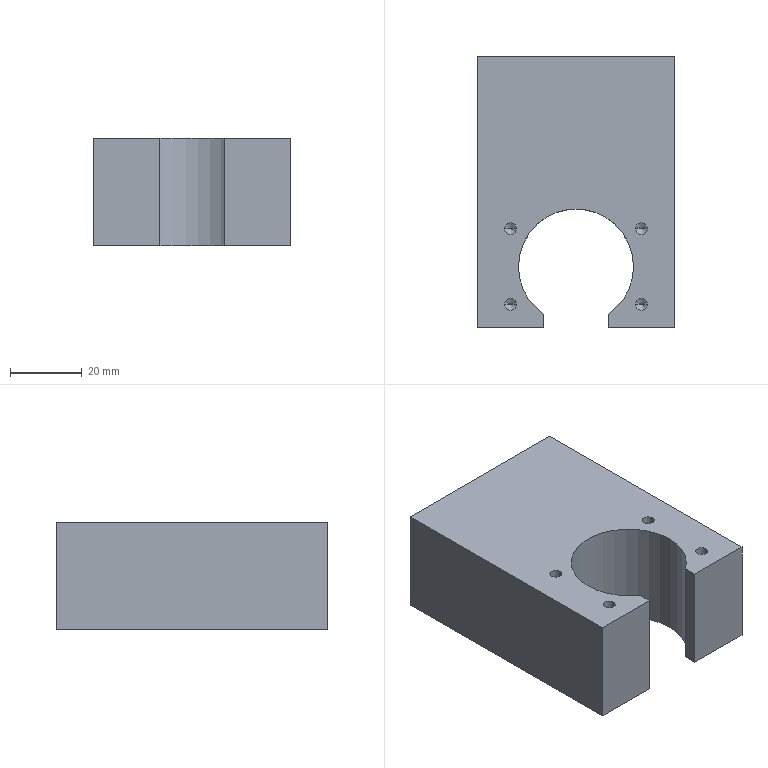Part | SolidWorks | features HoleWzd 2, 3DProfileFeature 1, Extrusion 1 | 1 solid | 52 faces | box 55 x 75.5 x 30 mm | volume 98100 mm3 | cone 24 | cylinder 19 | plane 9 | commonest cylinder face diameters 3.3 x8 5 x8 32 x3
STEP:
#1=CARTESIAN_POINT('',(-20.5,57.975,5.5));
#2=VERTEX_POINT('',#1);
#3=CARTESIAN_POINT('',(-20.5,57.975,10.5));
#4=VERTEX_POINT('',#3);
#5=CARTESIAN_POINT('',(-20.5,57.975,8.));
#6=DIRECTION('',(0.,1.,0.));
#7=DIRECTION('',(0.,0.,1.));
#8=AXIS2_PLACEMENT_3D('',#5,#6,#7);
#9=CIRCLE('',#8,2.5);
#10=EDGE_CURVE('',#2,#4,#9,.T.);
#11=ORIENTED_EDGE('',*,*,#10,.F.);
#12=CARTESIAN_POINT('',(-20.5,58.5,4.975));
#13=VERTEX_POINT('',#12);
#14=CARTESIAN_POINT('',(-20.5,58.5,4.975));
#15=DIRECTION('',(0.,0.7071,-0.7071));
#16=VECTOR('',#15,1000.);
#17=LINE('',#14,#16);
#18=EDGE_CURVE('',#2,#13,#17,.T.);
#19=ORIENTED_EDGE('',*,*,#18,.T.);
#20=CARTESIAN_POINT('',(-20.5,58.5,11.025));
#21=VERTEX_POINT('',#20);
#22=CARTESIAN_POINT('',(-20.5,58.5,8.));
#23=DIRECTION('',(0.,1.,0.));
#24=DIRECTION('',(0.,0.,1.));
#25=AXIS2_PLACEMENT_3D('',#22,#23,#24);
#26=CIRCLE('',#25,3.025);
#27=EDGE_CURVE('',#13,#21,#26,.T.);
#28=ORIENTED_EDGE('',*,*,#27,.T.);
#29=CARTESIAN_POINT('',(-20.5,58.5,11.025));
#30=DIRECTION('',(0.,0.7071,0.7071));
#31=VECTOR('',#30,1000.);
#32=LINE('',#29,#31);
#33=EDGE_CURVE('',#4,#21,#32,.T.);
#34=ORIENTED_EDGE('',*,*,#33,.F.);
#35=EDGE_LOOP('',(#11,#19,#28,#34));
#36=FACE_OUTER_BOUND('',#35,.T.);
#37=CARTESIAN_POINT('',(-20.5,58.5,8.));
#38=DIRECTION('',(0.,1.,0.));
#39=DIRECTION('',(0.,0.,1.));
#40=AXIS2_PLACEMENT_3D('',#37,#38,#39);
#41=CONICAL_SURFACE('',#40,3.025,0.7854);
#42=ADVANCED_FACE('',(#36),#41,.F.);
#43=CARTESIAN_POINT('',(-20.5,46.5,5.5));
#44=VERTEX_POINT('',#43);
#45=CARTESIAN_POINT('',(-20.5,46.5,10.5));
#46=VERTEX_POINT('',#45);
#47=CARTESIAN_POINT('',(-20.5,46.5,8.));
#48=DIRECTION('',(0.,1.,0.));
#49=DIRECTION('',(0.,0.,1.));
#50=AXIS2_PLACEMENT_3D('',#47,#48,#49);
#51=CIRCLE('',#50,2.5);
#52=EDGE_CURVE('',#44,#46,#51,.T.);
#53=ORIENTED_EDGE('',*,*,#52,.F.);
#54=CARTESIAN_POINT('',(-20.5,58.5,5.5));
#55=DIRECTION('',(0.,1.,0.));
#56=VECTOR('',#55,1000.);
#57=LINE('',#54,#56);
#58=EDGE_CURVE('',#44,#2,#57,.T.);
#59=ORIENTED_EDGE('',*,*,#58,.T.);
#60=ORIENTED_EDGE('',*,*,#10,.T.);
#61=CARTESIAN_POINT('',(-20.5,58.5,10.5));
#62=DIRECTION('',(0.,1.,0.));
#63=VECTOR('',#62,1000.);
#64=LINE('',#61,#63);
#65=EDGE_CURVE('',#46,#4,#64,.T.);
#66=ORIENTED_EDGE('',*,*,#65,.F.);
#67=EDGE_LOOP('',(#53,#59,#60,#66));
#68=FACE_OUTER_BOUND('',#67,.T.);
#69=CARTESIAN_POINT('',(-20.5,58.5,8.));
#70=DIRECTION('',(0.,1.,0.));
#71=DIRECTION('',(0.,0.,1.));
#72=AXIS2_PLACEMENT_3D('',#69,#70,#71);
#73=CYLINDRICAL_SURFACE('',#72,2.5);
#74=ADVANCED_FACE('',(#68),#73,.F.);
#75=CARTESIAN_POINT('',(-20.5,44.998,8.));
#76=VERTEX_POINT('',#75);
#77=CARTESIAN_POINT('',(-20.5,46.5,10.5));
#78=DIRECTION('',(0.,0.515,0.8572));
#79=VECTOR('',#78,1000.);
#80=LINE('',#77,#79);
#81=EDGE_CURVE('',#76,#46,#80,.T.);
#82=ORIENTED_EDGE('',*,*,#81,.F.);
#83=CARTESIAN_POINT('',(-20.5,46.5,5.5));
#84=DIRECTION('',(0.,0.515,-0.8572));
#85=VECTOR('',#84,1000.);
#86=LINE('',#83,#85);
#87=EDGE_CURVE('',#76,#44,#86,.T.);
#88=ORIENTED_EDGE('',*,*,#87,.T.);
#89=ORIENTED_EDGE('',*,*,#52,.T.);
#90=EDGE_LOOP('',(#82,#88,#89));
#91=FACE_OUTER_BOUND('',#90,.T.);
#92=CARTESIAN_POINT('',(-20.5,46.5,8.));
#93=DIRECTION('',(0.,1.,0.));
#94=DIRECTION('',(0.,0.,1.));
#95=AXIS2_PLACEMENT_3D('',#92,#93,#94);
#96=CONICAL_SURFACE('',#95,2.5,1.03);
#97=ADVANCED_FACE('',(#91),#96,.F.);
#98=CARTESIAN_POINT('',(-20.5,57.975,-10.5));
#99=VERTEX_POINT('',#98);
#100=CARTESIAN_POINT('',(-20.5,57.975,-5.5));
#101=VERTEX_POINT('',#100);
#102=CARTESIAN_POINT('',(-20.5,57.975,-8.));
#103=DIRECTION('',(0.,1.,0.));
#104=DIRECTION('',(0.,0.,1.));
#105=AXIS2_PLACEMENT_3D('',#102,#103,#104);
#106=CIRCLE('',#105,2.5);
#107=EDGE_CURVE('',#99,#101,#106,.T.);
#108=ORIENTED_EDGE('',*,*,#107,.F.);
#109=CARTESIAN_POINT('',(-20.5,58.5,-11.025));
#110=VERTEX_POINT('',#109);
#111=CARTESIAN_POINT('',(-20.5,58.5,-11.025));
#112=DIRECTION('',(0.,0.7071,-0.7071));
#113=VECTOR('',#112,1000.);
#114=LINE('',#111,#113);
#115=EDGE_CURVE('',#99,#110,#114,.T.);
#116=ORIENTED_EDGE('',*,*,#115,.T.);
#117=CARTESIAN_POINT('',(-20.5,58.5,-4.975));
#118=VERTEX_POINT('',#117);
#119=CARTESIAN_POINT('',(-20.5,58.5,-8.));
#120=DIRECTION('',(0.,1.,0.));
#121=DIRECTION('',(0.,0.,1.));
#122=AXIS2_PLACEMENT_3D('',#119,#120,#121);
#123=CIRCLE('',#122,3.025);
#124=EDGE_CURVE('',#110,#118,#123,.T.);
#125=ORIENTED_EDGE('',*,*,#124,.T.);
#126=CARTESIAN_POINT('',(-20.5,58.5,-4.975));
#127=DIRECTION('',(0.,0.7071,0.7071));
#128=VECTOR('',#127,1000.);
#129=LINE('',#126,#128);
#130=EDGE_CURVE('',#101,#118,#129,.T.);
#131=ORIENTED_EDGE('',*,*,#130,.F.);
#132=EDGE_LOOP('',(#108,#116,#125,#131));
#133=FACE_OUTER_BOUND('',#132,.T.);
#134=CARTESIAN_POINT('',(-20.5,58.5,-8.));
#135=DIRECTION('',(0.,1.,0.));
#136=DIRECTION('',(0.,0.,1.));
#137=AXIS2_PLACEMENT_3D('',#134,#135,#136);
#138=CONICAL_SURFACE('',#137,3.025,0.7854);
#139=ADVANCED_FACE('',(#133),#138,.F.);
#140=CARTESIAN_POINT('',(-20.5,46.5,-10.5));
#141=VERTEX_POINT('',#140);
#142=CARTESIAN_POINT('',(-20.5,46.5,-5.5));
#143=VERTEX_POINT('',#142);
#144=CARTESIAN_POINT('',(-20.5,46.5,-8.));
#145=DIRECTION('',(0.,1.,0.));
#146=DIRECTION('',(0.,0.,1.));
#147=AXIS2_PLACEMENT_3D('',#144,#145,#146);
#148=CIRCLE('',#147,2.5);
#149=EDGE_CURVE('',#141,#143,#148,.T.);
#150=ORIENTED_EDGE('',*,*,#149,.F.);
#151=CARTESIAN_POINT('',(-20.5,58.5,-10.5));
#152=DIRECTION('',(0.,1.,0.));
#153=VECTOR('',#152,1000.);
#154=LINE('',#151,#153);
#155=EDGE_CURVE('',#141,#99,#154,.T.);
#156=ORIENTED_EDGE('',*,*,#155,.T.);
#157=ORIENTED_EDGE('',*,*,#107,.T.);
#158=CARTESIAN_POINT('',(-20.5,58.5,-5.5));
#159=DIRECTION('',(0.,1.,0.));
#160=VECTOR('',#159,1000.);
#161=LINE('',#158,#160);
#162=EDGE_CURVE('',#143,#101,#161,.T.);
#163=ORIENTED_EDGE('',*,*,#162,.F.);
#164=EDGE_LOOP('',(#150,#156,#157,#163));
#165=FACE_OUTER_BOUND('',#164,.T.);
#166=CARTESIAN_POINT('',(-20.5,58.5,-8.));
#167=DIRECTION('',(0.,1.,0.));
#168=DIRECTION('',(0.,0.,1.));
#169=AXIS2_PLACEMENT_3D('',#166,#167,#168);
#170=CYLINDRICAL_SURFACE('',#169,2.5);
#171=ADVANCED_FACE('',(#165),#170,.F.);
#172=CARTESIAN_POINT('',(-20.5,44.998,-8.));
#173=VERTEX_POINT('',#172);
#174=CARTESIAN_POINT('',(-20.5,46.5,-5.5));
#175=DIRECTION('',(0.,0.515,0.8572));
#176=VECTOR('',#175,1000.);
#177=LINE('',#174,#176);
#178=EDGE_CURVE('',#173,#143,#177,.T.);
#179=ORIENTED_EDGE('',*,*,#178,.F.);
#180=CARTESIAN_POINT('',(-20.5,46.5,-10.5));
#181=DIRECTION('',(0.,0.515,-0.8572));
#182=VECTOR('',#181,1000.);
#183=LINE('',#180,#182);
#184=EDGE_CURVE('',#173,#141,#183,.T.);
#185=ORIENTED_EDGE('',*,*,#184,.T.);
#186=ORIENTED_EDGE('',*,*,#149,.T.);
#187=EDGE_LOOP('',(#179,#185,#186));
#188=FACE_OUTER_BOUND('',#187,.T.);
#189=CARTESIAN_POINT('',(-20.5,46.5,-8.));
#190=DIRECTION('',(0.,1.,0.));
#191=DIRECTION('',(0.,0.,1.));
#192=AXIS2_PLACEMENT_3D('',#189,#190,#191);
#193=CONICAL_SURFACE('',#192,2.5,1.03);
#194=ADVANCED_FACE('',(#188),#193,.F.);
#195=CARTESIAN_POINT('',(20.5,57.975,-10.5));
#196=VERTEX_POINT('',#195);
#197=CARTESIAN_POINT('',(20.5,57.975,-5.5));
#198=VERTEX_POINT('',#197);
#199=CARTESIAN_POINT('',(20.5,57.975,-8.));
#200=DIRECTION('',(0.,1.,0.));
#201=DIRECTION('',(0.,0.,1.));
#202=AXIS2_PLACEMENT_3D('',#199,#200,#201);
#203=CIRCLE('',#202,2.5);
#204=EDGE_CURVE('',#196,#198,#203,.T.);
#205=ORIENTED_EDGE('',*,*,#204,.F.);
#206=CARTESIAN_POINT('',(20.5,58.5,-11.025));
#207=VERTEX_POINT('',#206);
#208=CARTESIAN_POINT('',(20.5,58.5,-11.025));
#209=DIRECTION('',(0.,0.7071,-0.7071));
#210=VECTOR('',#209,1000.);
#211=LINE('',#208,#210);
#212=EDGE_CURVE('',#196,#207,#211,.T.);
#213=ORIENTED_EDGE('',*,*,#212,.T.);
#214=CARTESIAN_POINT('',(20.5,58.5,-4.975));
#215=VERTEX_POINT('',#214);
#216=CARTESIAN_POINT('',(20.5,58.5,-8.));
#217=DIRECTION('',(0.,1.,0.));
#218=DIRECTION('',(0.,0.,1.));
#219=AXIS2_PLACEMENT_3D('',#216,#217,#218);
#220=CIRCLE('',#219,3.025);
#221=EDGE_CURVE('',#207,#215,#220,.T.);
#222=ORIENTED_EDGE('',*,*,#221,.T.);
#223=CARTESIAN_POINT('',(20.5,58.5,-4.975));
#224=DIRECTION('',(0.,0.7071,0.7071));
#225=VECTOR('',#224,1000.);
#226=LINE('',#223,#225);
#227=EDGE_CURVE('',#198,#215,#226,.T.);
#228=ORIENTED_EDGE('',*,*,#227,.F.);
#229=EDGE_LOOP('',(#205,#213,#222,#228));
#230=FACE_OUTER_BOUND('',#229,.T.);
#231=CARTESIAN_POINT('',(20.5,58.5,-8.));
#232=DIRECTION('',(0.,1.,0.));
#233=DIRECTION('',(0.,0.,1.));
#234=AXIS2_PLACEMENT_3D('',#231,#232,#233);
#235=CONICAL_SURFACE('',#234,3.025,0.7854);
#236=ADVANCED_FACE('',(#230),#235,.F.);
#237=CARTESIAN_POINT('',(20.5,46.5,-10.5));
#238=VERTEX_POINT('',#237);
#239=CARTESIAN_POINT('',(20.5,46.5,-5.5));
#240=VERTEX_POINT('',#239);
#241=CARTESIAN_POINT('',(20.5,46.5,-8.));
#242=DIRECTION('',(0.,1.,0.));
#243=DIRECTION('',(0.,0.,1.));
#244=AXIS2_PLACEMENT_3D('',#241,#242,#243);
#245=CIRCLE('',#244,2.5);
#246=EDGE_CURVE('',#238,#240,#245,.T.);
#247=ORIENTED_EDGE('',*,*,#246,.F.);
#248=CARTESIAN_POINT('',(20.5,58.5,-10.5));
#249=DIRECTION('',(0.,1.,0.));
#250=VECTOR('',#249,1000.);
#251=LINE('',#248,#250);
#252=EDGE_CURVE('',#238,#196,#251,.T.);
#253=ORIENTED_EDGE('',*,*,#252,.T.);
#254=ORIENTED_EDGE('',*,*,#204,.T.);
#255=CARTESIAN_POINT('',(20.5,58.5,-5.5));
#256=DIRECTION('',(0.,1.,0.));
#257=VECTOR('',#256,1000.);
#258=LINE('',#255,#257);
#259=EDGE_CURVE('',#240,#198,#258,.T.);
#260=ORIENTED_EDGE('',*,*,#259,.F.);
#261=EDGE_LOOP('',(#247,#253,#254,#260));
#262=FACE_OUTER_BOUND('',#261,.T.);
#263=CARTESIAN_POINT('',(20.5,58.5,-8.));
#264=DIRECTION('',(0.,1.,0.));
#265=DIRECTION('',(0.,0.,1.));
#266=AXIS2_PLACEMENT_3D('',#263,#264,#265);
#267=CYLINDRICAL_SURFACE('',#266,2.5);
#268=ADVANCED_FACE('',(#262),#267,.F.);
#269=CARTESIAN_POINT('',(20.5,44.998,-8.));
#270=VERTEX_POINT('',#269);
#271=CARTESIAN_POINT('',(20.5,46.5,-5.5));
#272=DIRECTION('',(0.,0.515,0.8572));
#273=VECTOR('',#272,1000.);
#274=LINE('',#271,#273);
#275=EDGE_CURVE('',#270,#240,#274,.T.);
#276=ORIENTED_EDGE('',*,*,#275,.F.);
#277=CARTESIAN_POINT('',(20.5,46.5,-10.5));
#278=DIRECTION('',(0.,0.515,-0.8572));
#279=VECTOR('',#278,1000.);
#280=LINE('',#277,#279);
#281=EDGE_CURVE('',#270,#238,#280,.T.);
#282=ORIENTED_EDGE('',*,*,#281,.T.);
#283=ORIENTED_EDGE('',*,*,#246,.T.);
#284=EDGE_LOOP('',(#276,#282,#283));
#285=FACE_OUTER_BOUND('',#284,.T.);
#286=CARTESIAN_POINT('',(20.5,46.5,-8.));
#287=DIRECTION('',(0.,1.,0.));
#288=DIRECTION('',(0.,0.,1.));
#289=AXIS2_PLACEMENT_3D('',#286,#287,#288);
#290=CONICAL_SURFACE('',#289,2.5,1.03);
#291=ADVANCED_FACE('',(#285),#290,.F.);
#292=CARTESIAN_POINT('',(20.5,57.975,5.5));
#293=VERTEX_POINT('',#292);
#294=CARTESIAN_POINT('',(20.5,57.975,10.5));
#295=VERTEX_POINT('',#294);
#296=CARTESIAN_POINT('',(20.5,57.975,8.));
#297=DIRECTION('',(0.,1.,0.));
#298=DIRECTION('',(0.,0.,1.));
#299=AXIS2_PLACEMENT_3D('',#296,#297,#298);
#300=CIRCLE('',#299,2.5);
#301=EDGE_CURVE('',#293,#295,#300,.T.);
#302=ORIENTED_EDGE('',*,*,#301,.F.);
#303=CARTESIAN_POINT('',(20.5,58.5,4.975));
#304=VERTEX_POINT('',#303);
#305=CARTESIAN_POINT('',(20.5,58.5,4.975));
#306=DIRECTION('',(0.,0.7071,-0.7071));
#307=VECTOR('',#306,1000.);
#308=LINE('',#305,#307);
#309=EDGE_CURVE('',#293,#304,#308,.T.);
#310=ORIENTED_EDGE('',*,*,#309,.T.);
#311=CARTESIAN_POINT('',(20.5,58.5,11.025));
#312=VERTEX_POINT('',#311);
#313=CARTESIAN_POINT('',(20.5,58.5,8.));
#314=DIRECTION('',(0.,1.,0.));
#315=DIRECTION('',(0.,0.,1.));
#316=AXIS2_PLACEMENT_3D('',#313,#314,#315);
#317=CIRCLE('',#316,3.025);
#318=EDGE_CURVE('',#304,#312,#317,.T.);
#319=ORIENTED_EDGE('',*,*,#318,.T.);
#320=CARTESIAN_POINT('',(20.5,58.5,11.025));
#321=DIRECTION('',(0.,0.7071,0.7071));
#322=VECTOR('',#321,1000.);
#323=LINE('',#320,#322);
#324=EDGE_CURVE('',#295,#312,#323,.T.);
#325=ORIENTED_EDGE('',*,*,#324,.F.);
#326=EDGE_LOOP('',(#302,#310,#319,#325));
#327=FACE_OUTER_BOUND('',#326,.T.);
#328=CARTESIAN_POINT('',(20.5,58.5,8.));
#329=DIRECTION('',(0.,1.,0.));
#330=DIRECTION('',(0.,0.,1.));
#331=AXIS2_PLACEMENT_3D('',#328,#329,#330);
#332=CONICAL_SURFACE('',#331,3.025,0.7854);
#333=ADVANCED_FACE('',(#327),#332,.F.);
#334=CARTESIAN_POINT('',(20.5,46.5,5.5));
#335=VERTEX_POINT('',#334);
#336=CARTESIAN_POINT('',(20.5,46.5,10.5));
#337=VERTEX_POINT('',#336);
#338=CARTESIAN_POINT('',(20.5,46.5,8.));
#339=DIRECTION('',(0.,1.,0.));
#340=DIRECTION('',(0.,0.,1.));
#341=AXIS2_PLACEMENT_3D('',#338,#339,#340);
#342=CIRCLE('',#341,2.5);
#343=EDGE_CURVE('',#335,#337,#342,.T.);
#344=ORIENTED_EDGE('',*,*,#343,.F.);
#345=CARTESIAN_POINT('',(20.5,58.5,5.5));
#346=DIRECTION('',(0.,1.,0.));
#347=VECTOR('',#346,1000.);
#348=LINE('',#345,#347);
#349=EDGE_CURVE('',#335,#293,#348,.T.);
#350=ORIENTED_EDGE('',*,*,#349,.T.);
#351=ORIENTED_EDGE('',*,*,#301,.T.);
#352=CARTESIAN_POINT('',(20.5,58.5,10.5));
#353=DIRECTION('',(0.,1.,0.));
#354=VECTOR('',#353,1000.);
#355=LINE('',#352,#354);
#356=EDGE_CURVE('',#337,#295,#355,.T.);
#357=ORIENTED_EDGE('',*,*,#356,.F.);
#358=EDGE_LOOP('',(#344,#350,#351,#357));
#359=FACE_OUTER_BOUND('',#358,.T.);
#360=CARTESIAN_POINT('',(20.5,58.5,8.));
#361=DIRECTION('',(0.,1.,0.));
#362=DIRECTION('',(0.,0.,1.));
#363=AXIS2_PLACEMENT_3D('',#360,#361,#362);
#364=CYLINDRICAL_SURFACE('',#363,2.5);
#365=ADVANCED_FACE('',(#359),#364,.F.);
#366=CARTESIAN_POINT('',(20.5,44.998,8.));
#367=VERTEX_POINT('',#366);
#368=CARTESIAN_POINT('',(20.5,46.5,10.5));
#369=DIRECTION('',(0.,0.515,0.8572));
#370=VECTOR('',#369,1000.);
#371=LINE('',#368,#370);
#372=EDGE_CURVE('',#367,#337,#371,.T.);
#373=ORIENTED_EDGE('',*,*,#372,.F.);
#374=CARTESIAN_POINT('',(20.5,46.5,5.5));
#375=DIRECTION('',(0.,0.515,-0.8572));
#376=VECTOR('',#375,1000.);
#377=LINE('',#374,#376);
#378=EDGE_CURVE('',#367,#335,#377,.T.);
#379=ORIENTED_EDGE('',*,*,#378,.T.);
#380=ORIENTED_EDGE('',*,*,#343,.T.);
#381=EDGE_LOOP('',(#373,#379,#380));
#382=FACE_OUTER_BOUND('',#381,.T.);
#383=CARTESIAN_POINT('',(20.5,46.5,8.));
#384=DIRECTION('',(0.,1.,0.));
#385=DIRECTION('',(0.,0.,1.));
#386=AXIS2_PLACEMENT_3D('',#383,#384,#385);
#387=CONICAL_SURFACE('',#386,2.5,1.03);
#388=ADVANCED_FACE('',(#382),#387,.F.);
#389=CARTESIAN_POINT('',(16.537,10.5,5.5));
#390=VERTEX_POINT('',#389);
#391=CARTESIAN_POINT('',(19.837,10.5,5.5));
#392=VERTEX_POINT('',#391);
#393=CARTESIAN_POINT('',(18.187,10.5,5.5));
#394=DIRECTION('',(0.,0.,1.));
#395=DIRECTION('',(1.,0.,0.));
#396=AXIS2_PLACEMENT_3D('',#393,#394,#395);
#397=CIRCLE('',#396,1.65);
#398=EDGE_CURVE('',#390,#392,#397,.T.);
#399=ORIENTED_EDGE('',*,*,#398,.F.);
#400=CARTESIAN_POINT('',(16.537,10.5,15.));
#401=VERTEX_POINT('',#400);
#402=CARTESIAN_POINT('',(16.537,10.5,15.));
#403=DIRECTION('',(0.,0.,1.));
#404=VECTOR('',#403,1000.);
#405=LINE('',#402,#404);
#406=EDGE_CURVE('',#390,#401,#405,.T.);
#407=ORIENTED_EDGE('',*,*,#406,.T.);
#408=CARTESIAN_POINT('',(19.837,10.5,15.));
#409=VERTEX_POINT('',#408);
#410=CARTESIAN_POINT('',(18.187,10.5,15.));
#411=DIRECTION('',(0.,0.,1.));
#412=DIRECTION('',(1.,0.,0.));
#413=AXIS2_PLACEMENT_3D('',#410,#411,#412);
#414=CIRCLE('',#413,1.65);
#415=EDGE_CURVE('',#401,#409,#414,.T.);
#416=ORIENTED_EDGE('',*,*,#415,.T.);
#417=CARTESIAN_POINT('',(19.837,10.5,15.));
#418=DIRECTION('',(0.,0.,1.));
#419=VECTOR('',#418,1000.);
#420=LINE('',#417,#419);
#421=EDGE_CURVE('',#392,#409,#420,.T.);
#422=ORIENTED_EDGE('',*,*,#421,.F.);
#423=EDGE_LOOP('',(#399,#407,#416,#422));
#424=FACE_OUTER_BOUND('',#423,.T.);
#425=CARTESIAN_POINT('',(18.187,10.5,15.));
#426=DIRECTION('',(0.,0.,1.));
#427=DIRECTION('',(1.,0.,0.));
#428=AXIS2_PLACEMENT_3D('',#425,#426,#427);
#429=CYLINDRICAL_SURFACE('',#428,1.65);
#430=ADVANCED_FACE('',(#424),#429,.F.);
#431=CARTESIAN_POINT('',(18.187,10.5,4.509));
#432=VERTEX_POINT('',#431);
#433=CARTESIAN_POINT('',(19.837,10.5,5.5));
#434=DIRECTION('',(0.8572,0.,0.515));
#435=VECTOR('',#434,1000.);
#436=LINE('',#433,#435);
#437=EDGE_CURVE('',#432,#392,#436,.T.);
#438=ORIENTED_EDGE('',*,*,#437,.F.);
#439=CARTESIAN_POINT('',(16.537,10.5,5.5));
#440=DIRECTION('',(-0.8572,0.,0.515));
#441=VECTOR('',#440,1000.);
#442=LINE('',#439,#441);
#443=EDGE_CURVE('',#432,#390,#442,.T.);
#444=ORIENTED_EDGE('',*,*,#443,.T.);
#445=ORIENTED_EDGE('',*,*,#398,.T.);
#446=EDGE_LOOP('',(#438,#444,#445));
#447=FACE_OUTER_BOUND('',#446,.T.);
#448=CARTESIAN_POINT('',(18.187,10.5,5.5));
#449=DIRECTION('',(0.,0.,1.));
#450=DIRECTION('',(1.,0.,0.));
#451=AXIS2_PLACEMENT_3D('',#448,#449,#450);
#452=CONICAL_SURFACE('',#451,1.65,1.03);
#453=ADVANCED_FACE('',(#447),#452,.F.);
#454=CARTESIAN_POINT('',(16.537,-10.5,5.5));
#455=VERTEX_POINT('',#454);
#456=CARTESIAN_POINT('',(19.837,-10.5,5.5));
#457=VERTEX_POINT('',#456);
#458=CARTESIAN_POINT('',(18.187,-10.5,5.5));
#459=DIRECTION('',(0.,0.,1.));
#460=DIRECTION('',(1.,0.,0.));
#461=AXIS2_PLACEMENT_3D('',#458,#459,#460);
#462=CIRCLE('',#461,1.65);
#463=EDGE_CURVE('',#455,#457,#462,.T.);
#464=ORIENTED_EDGE('',*,*,#463,.F.);
#465=CARTESIAN_POINT('',(16.537,-10.5,15.));
#466=VERTEX_POINT('',#465);
#467=CARTESIAN_POINT('',(16.537,-10.5,15.));
#468=DIRECTION('',(0.,0.,1.));
#469=VECTOR('',#468,1000.);
#470=LINE('',#467,#469);
#471=EDGE_CURVE('',#455,#466,#470,.T.);
#472=ORIENTED_EDGE('',*,*,#471,.T.);
#473=CARTESIAN_POINT('',(19.837,-10.5,15.));
#474=VERTEX_POINT('',#473);
#475=CARTESIAN_POINT('',(18.187,-10.5,15.));
#476=DIRECTION('',(0.,0.,1.));
#477=DIRECTION('',(1.,0.,0.));
#478=AXIS2_PLACEMENT_3D('',#475,#476,#477);
#479=CIRCLE('',#478,1.65);
#480=EDGE_CURVE('',#466,#474,#479,.T.);
#481=ORIENTED_EDGE('',*,*,#480,.T.);
#482=CARTESIAN_POINT('',(19.837,-10.5,15.));
#483=DIRECTION('',(0.,0.,1.));
#484=VECTOR('',#483,1000.);
#485=LINE('',#482,#484);
#486=EDGE_CURVE('',#457,#474,#485,.T.);
#487=ORIENTED_EDGE('',*,*,#486,.F.);
#488=EDGE_LOOP('',(#464,#472,#481,#487));
#489=FACE_OUTER_BOUND('',#488,.T.);
#490=CARTESIAN_POINT('',(18.187,-10.5,15.));
#491=DIRECTION('',(0.,0.,1.));
#492=DIRECTION('',(1.,0.,0.));
#493=AXIS2_PLACEMENT_3D('',#490,#491,#492);
#494=CYLINDRICAL_SURFACE('',#493,1.65);
#495=ADVANCED_FACE('',(#489),#494,.F.);
#496=CARTESIAN_POINT('',(18.187,-10.5,4.509));
#497=VERTEX_POINT('',#496);
#498=CARTESIAN_POINT('',(19.837,-10.5,5.5));
#499=DIRECTION('',(0.8572,0.,0.515));
#500=VECTOR('',#499,1000.);
#501=LINE('',#498,#500);
#502=EDGE_CURVE('',#497,#457,#501,.T.);
#503=ORIENTED_EDGE('',*,*,#502,.F.);
#504=CARTESIAN_POINT('',(16.537,-10.5,5.5));
#505=DIRECTION('',(-0.8572,0.,0.515));
#506=VECTOR('',#505,1000.);
#507=LINE('',#504,#506);
#508=EDGE_CURVE('',#497,#455,#507,.T.);
#509=ORIENTED_EDGE('',*,*,#508,.T.);
#510=ORIENTED_EDGE('',*,*,#463,.T.);
#511=EDGE_LOOP('',(#503,#509,#510));
#512=FACE_OUTER_BOUND('',#511,.T.);
#513=CARTESIAN_POINT('',(18.187,-10.5,5.5));
#514=DIRECTION('',(0.,0.,1.));
#515=DIRECTION('',(1.,0.,0.));
#516=AXIS2_PLACEMENT_3D('',#513,#514,#515);
#517=CONICAL_SURFACE('',#516,1.65,1.03);
#518=ADVANCED_FACE('',(#512),#517,.F.);
#519=CARTESIAN_POINT('',(-19.837,-10.5,5.5));
#520=VERTEX_POINT('',#519);
#521=CARTESIAN_POINT('',(-16.537,-10.5,5.5));
#522=VERTEX_POINT('',#521);
#523=CARTESIAN_POINT('',(-18.187,-10.5,5.5));
#524=DIRECTION('',(0.,0.,1.));
#525=DIRECTION('',(1.,0.,0.));
#526=AXIS2_PLACEMENT_3D('',#523,#524,#525);
#527=CIRCLE('',#526,1.65);
#528=EDGE_CURVE('',#520,#522,#527,.T.);
#529=ORIENTED_EDGE('',*,*,#528,.F.);
#530=CARTESIAN_POINT('',(-19.837,-10.5,15.));
#531=VERTEX_POINT('',#530);
#532=CARTESIAN_POINT('',(-19.837,-10.5,15.));
#533=DIRECTION('',(0.,0.,1.));
#534=VECTOR('',#533,1000.);
#535=LINE('',#532,#534);
#536=EDGE_CURVE('',#520,#531,#535,.T.);
#537=ORIENTED_EDGE('',*,*,#536,.T.);
#538=CARTESIAN_POINT('',(-16.537,-10.5,15.));
#539=VERTEX_POINT('',#538);
#540=CARTESIAN_POINT('',(-18.187,-10.5,15.));
#541=DIRECTION('',(0.,0.,1.));
#542=DIRECTION('',(1.,0.,0.));
#543=AXIS2_PLACEMENT_3D('',#540,#541,#542);
#544=CIRCLE('',#543,1.65);
#545=EDGE_CURVE('',#531,#539,#544,.T.);
#546=ORIENTED_EDGE('',*,*,#545,.T.);
#547=CARTESIAN_POINT('',(-16.537,-10.5,15.));
#548=DIRECTION('',(0.,0.,1.));
#549=VECTOR('',#548,1000.);
#550=LINE('',#547,#549);
#551=EDGE_CURVE('',#522,#539,#550,.T.);
#552=ORIENTED_EDGE('',*,*,#551,.F.);
#553=EDGE_LOOP('',(#529,#537,#546,#552));
#554=FACE_OUTER_BOUND('',#553,.T.);
#555=CARTESIAN_POINT('',(-18.187,-10.5,15.));
#556=DIRECTION('',(0.,0.,1.));
#557=DIRECTION('',(1.,0.,0.));
#558=AXIS2_PLACEMENT_3D('',#555,#556,#557);
#559=CYLINDRICAL_SURFACE('',#558,1.65);
#560=ADVANCED_FACE('',(#554),#559,.F.);
#561=CARTESIAN_POINT('',(-18.187,-10.5,4.509));
#562=VERTEX_POINT('',#561);
#563=CARTESIAN_POINT('',(-16.537,-10.5,5.5));
#564=DIRECTION('',(0.8572,0.,0.515));
#565=VECTOR('',#564,1000.);
#566=LINE('',#563,#565);
#567=EDGE_CURVE('',#562,#522,#566,.T.);
#568=ORIENTED_EDGE('',*,*,#567,.F.);
#569=CARTESIAN_POINT('',(-19.837,-10.5,5.5));
#570=DIRECTION('',(-0.8572,0.,0.515));
#571=VECTOR('',#570,1000.);
#572=LINE('',#569,#571);
#573=EDGE_CURVE('',#562,#520,#572,.T.);
#574=ORIENTED_EDGE('',*,*,#573,.T.);
#575=ORIENTED_EDGE('',*,*,#528,.T.);
#576=EDGE_LOOP('',(#568,#574,#575));
#577=FACE_OUTER_BOUND('',#576,.T.);
#578=CARTESIAN_POINT('',(-18.187,-10.5,5.5));
#579=DIRECTION('',(0.,0.,1.));
#580=DIRECTION('',(1.,0.,0.));
#581=AXIS2_PLACEMENT_3D('',#578,#579,#580);
#582=CONICAL_SURFACE('',#581,1.65,1.03);
#583=ADVANCED_FACE('',(#577),#582,.F.);
#584=CARTESIAN_POINT('',(-19.837,10.5,5.5));
#585=VERTEX_POINT('',#584);
#586=CARTESIAN_POINT('',(-16.537,10.5,5.5));
#587=VERTEX_POINT('',#586);
#588=CARTESIAN_POINT('',(-18.187,10.5,5.5));
#589=DIRECTION('',(0.,0.,1.));
#590=DIRECTION('',(1.,0.,0.));
#591=AXIS2_PLACEMENT_3D('',#588,#589,#590);
#592=CIRCLE('',#591,1.65);
#593=EDGE_CURVE('',#585,#587,#592,.T.);
#594=ORIENTED_EDGE('',*,*,#593,.F.);
#595=CARTESIAN_POINT('',(-19.837,10.5,15.));
#596=VERTEX_POINT('',#595);
#597=CARTESIAN_POINT('',(-19.837,10.5,15.));
#598=DIRECTION('',(0.,0.,1.));
#599=VECTOR('',#598,1000.);
#600=LINE('',#597,#599);
#601=EDGE_CURVE('',#585,#596,#600,.T.);
#602=ORIENTED_EDGE('',*,*,#601,.T.);
#603=CARTESIAN_POINT('',(-16.537,10.5,15.));
#604=VERTEX_POINT('',#603);
#605=CARTESIAN_POINT('',(-18.187,10.5,15.));
#606=DIRECTION('',(0.,0.,1.));
#607=DIRECTION('',(1.,0.,0.));
#608=AXIS2_PLACEMENT_3D('',#605,#606,#607);
#609=CIRCLE('',#608,1.65);
#610=EDGE_CURVE('',#596,#604,#609,.T.);
#611=ORIENTED_EDGE('',*,*,#610,.T.);
#612=CARTESIAN_POINT('',(-16.537,10.5,15.));
#613=DIRECTION('',(0.,0.,1.));
#614=VECTOR('',#613,1000.);
#615=LINE('',#612,#614);
#616=EDGE_CURVE('',#587,#604,#615,.T.);
#617=ORIENTED_EDGE('',*,*,#616,.F.);
#618=EDGE_LOOP('',(#594,#602,#611,#617));
#619=FACE_OUTER_BOUND('',#618,.T.);
#620=CARTESIAN_POINT('',(-18.187,10.5,15.));
#621=DIRECTION('',(0.,0.,1.));
#622=DIRECTION('',(1.,0.,0.));
#623=AXIS2_PLACEMENT_3D('',#620,#621,#622);
#624=CYLINDRICAL_SURFACE('',#623,1.65);
#625=ADVANCED_FACE('',(#619),#624,.F.);
#626=CARTESIAN_POINT('',(-18.187,10.5,4.509));
#627=VERTEX_POINT('',#626);
#628=CARTESIAN_POINT('',(-16.537,10.5,5.5));
#629=DIRECTION('',(0.8572,0.,0.515));
#630=VECTOR('',#629,1000.);
#631=LINE('',#628,#630);
#632=EDGE_CURVE('',#627,#587,#631,.T.);
#633=ORIENTED_EDGE('',*,*,#632,.F.);
#634=CARTESIAN_POINT('',(-19.837,10.5,5.5));
#635=DIRECTION('',(-0.8572,0.,0.515));
#636=VECTOR('',#635,1000.);
#637=LINE('',#634,#636);
#638=EDGE_CURVE('',#627,#585,#637,.T.);
#639=ORIENTED_EDGE('',*,*,#638,.T.);
#640=ORIENTED_EDGE('',*,*,#593,.T.);
#641=EDGE_LOOP('',(#633,#639,#640));
#642=FACE_OUTER_BOUND('',#641,.T.);
#643=CARTESIAN_POINT('',(-18.187,10.5,5.5));
#644=DIRECTION('',(0.,0.,1.));
#645=DIRECTION('',(1.,0.,0.));
#646=AXIS2_PLACEMENT_3D('',#643,#644,#645);
#647=CONICAL_SURFACE('',#646,1.65,1.03);
#648=ADVANCED_FACE('',(#642),#647,.F.);
#649=CARTESIAN_POINT('',(16.,0.,15.));
#650=VERTEX_POINT('',#649);
#651=CARTESIAN_POINT('',(9.,-13.229,15.));
#652=VERTEX_POINT('',#651);
#653=CARTESIAN_POINT('',(0.,0.,15.));
#654=DIRECTION('',(0.,0.,-1.));
#655=DIRECTION('',(1.,0.,0.));
#656=AXIS2_PLACEMENT_3D('',#653,#654,#655);
#657=CIRCLE('',#656,16.);
#658=EDGE_CURVE('',#650,#652,#657,.T.);
#659=ORIENTED_EDGE('',*,*,#658,.F.);
#660=CARTESIAN_POINT('',(16.,0.,-15.));
#661=VERTEX_POINT('',#660);
#662=CARTESIAN_POINT('',(16.,0.,15.));
#663=DIRECTION('',(0.,0.,-1.));
#664=VECTOR('',#663,1000.);
#665=LINE('',#662,#664);
#666=EDGE_CURVE('',#650,#661,#665,.T.);
#667=ORIENTED_EDGE('',*,*,#666,.T.);
#668=CARTESIAN_POINT('',(9.,-13.229,-15.));
#669=VERTEX_POINT('',#668);
#670=CARTESIAN_POINT('',(0.,0.,-15.));
#671=DIRECTION('',(0.,0.,-1.));
#672=DIRECTION('',(1.,0.,0.));
#673=AXIS2_PLACEMENT_3D('',#670,#671,#672);
#674=CIRCLE('',#673,16.);
#675=EDGE_CURVE('',#661,#669,#674,.T.);
#676=ORIENTED_EDGE('',*,*,#675,.T.);
#677=CARTESIAN_POINT('',(9.,-13.229,15.));
#678=DIRECTION('',(0.,0.,-1.));
#679=VECTOR('',#678,1000.);
#680=LINE('',#677,#679);
#681=EDGE_CURVE('',#652,#669,#680,.T.);
#682=ORIENTED_EDGE('',*,*,#681,.F.);
#683=EDGE_LOOP('',(#659,#667,#676,#682));
#684=FACE_OUTER_BOUND('',#683,.T.);
#685=CARTESIAN_POINT('',(0.,0.,15.));
#686=DIRECTION('',(0.,0.,-1.));
#687=DIRECTION('',(-1.,0.,0.));
#688=AXIS2_PLACEMENT_3D('',#685,#686,#687);
#689=CYLINDRICAL_SURFACE('',#688,16.);
#690=ADVANCED_FACE('',(#684),#689,.F.);
#691=ORIENTED_EDGE('',*,*,#666,.F.);
#692=CARTESIAN_POINT('',(-16.,0.,15.));
#693=VERTEX_POINT('',#692);
#694=CARTESIAN_POINT('',(0.,0.,15.));
#695=DIRECTION('',(0.,0.,-1.));
#696=DIRECTION('',(1.,0.,0.));
#697=AXIS2_PLACEMENT_3D('',#694,#695,#696);
#698=CIRCLE('',#697,16.);
#699=EDGE_CURVE('',#693,#650,#698,.T.);
#700=ORIENTED_EDGE('',*,*,#699,.F.);
#701=CARTESIAN_POINT('',(-16.,0.,-15.));
#702=VERTEX_POINT('',#701);
#703=CARTESIAN_POINT('',(-16.,0.,15.));
#704=DIRECTION('',(0.,0.,-1.));
#705=VECTOR('',#704,1000.);
#706=LINE('',#703,#705);
#707=EDGE_CURVE('',#693,#702,#706,.T.);
#708=ORIENTED_EDGE('',*,*,#707,.T.);
#709=CARTESIAN_POINT('',(0.,0.,-15.));
#710=DIRECTION('',(0.,0.,-1.));
#711=DIRECTION('',(1.,0.,0.));
#712=AXIS2_PLACEMENT_3D('',#709,#710,#711);
#713=CIRCLE('',#712,16.);
#714=EDGE_CURVE('',#702,#661,#713,.T.);
#715=ORIENTED_EDGE('',*,*,#714,.T.);
#716=EDGE_LOOP('',(#691,#700,#708,#715));
#717=FACE_OUTER_BOUND('',#716,.T.);
#718=CARTESIAN_POINT('',(0.,0.,15.));
#719=DIRECTION('',(0.,0.,-1.));
#720=DIRECTION('',(-1.,0.,0.));
#721=AXIS2_PLACEMENT_3D('',#718,#719,#720);
#722=CYLINDRICAL_SURFACE('',#721,16.);
#723=ADVANCED_FACE('',(#717),#722,.F.);
#724=CARTESIAN_POINT('',(-27.5,58.5,-15.));
#725=VERTEX_POINT('',#724);
#726=CARTESIAN_POINT('',(-27.5,-17.,-15.));
#727=VERTEX_POINT('',#726);
#728=CARTESIAN_POINT('',(-27.5,58.5,-15.));
#729=DIRECTION('',(0.,-1.,0.));
#730=VECTOR('',#729,1000.);
#731=LINE('',#728,#730);
#732=EDGE_CURVE('',#725,#727,#731,.T.);
#733=ORIENTED_EDGE('',*,*,#732,.T.);
#734=CARTESIAN_POINT('',(-27.5,-17.,15.));
#735=VERTEX_POINT('',#734);
#736=CARTESIAN_POINT('',(-27.5,-17.,15.));
#737=DIRECTION('',(0.,0.,-1.));
#738=VECTOR('',#737,1000.);
#739=LINE('',#736,#738);
#740=EDGE_CURVE('',#735,#727,#739,.T.);
#741=ORIENTED_EDGE('',*,*,#740,.F.);
#742=CARTESIAN_POINT('',(-27.5,58.5,15.));
#743=VERTEX_POINT('',#742);
#744=CARTESIAN_POINT('',(-27.5,58.5,15.));
#745=DIRECTION('',(0.,-1.,0.));
#746=VECTOR('',#745,1000.);
#747=LINE('',#744,#746);
#748=EDGE_CURVE('',#743,#735,#747,.T.);
#749=ORIENTED_EDGE('',*,*,#748,.F.);
#750=CARTESIAN_POINT('',(-27.5,58.5,15.));
#751=DIRECTION('',(0.,0.,-1.));
#752=VECTOR('',#751,1000.);
#753=LINE('',#750,#752);
#754=EDGE_CURVE('',#743,#725,#753,.T.);
#755=ORIENTED_EDGE('',*,*,#754,.T.);
#756=EDGE_LOOP('',(#733,#741,#749,#755));
#757=FACE_OUTER_BOUND('',#756,.T.);
#758=CARTESIAN_POINT('',(-27.5,58.5,15.));
#759=DIRECTION('',(1.,0.,0.));
#760=DIRECTION('',(0.,0.,-1.));
#761=AXIS2_PLACEMENT_3D('',#758,#759,#760);
#762=PLANE('',#761);
#763=ADVANCED_FACE('',(#757),#762,.F.);
#764=CARTESIAN_POINT('',(-9.,-17.,-15.));
#765=VERTEX_POINT('',#764);
#766=CARTESIAN_POINT('',(-27.5,-17.,-15.));
#767=DIRECTION('',(1.,0.,0.));
#768=VECTOR('',#767,1000.);
#769=LINE('',#766,#768);
#770=EDGE_CURVE('',#727,#765,#769,.T.);
#771=ORIENTED_EDGE('',*,*,#770,.T.);
#772=CARTESIAN_POINT('',(-9.,-17.,15.));
#773=VERTEX_POINT('',#772);
#774=CARTESIAN_POINT('',(-9.,-17.,15.));
#775=DIRECTION('',(0.,0.,-1.));
#776=VECTOR('',#775,1000.);
#777=LINE('',#774,#776);
#778=EDGE_CURVE('',#773,#765,#777,.T.);
#779=ORIENTED_EDGE('',*,*,#778,.F.);
#780=CARTESIAN_POINT('',(-27.5,-17.,15.));
#781=DIRECTION('',(1.,0.,0.));
#782=VECTOR('',#781,1000.);
#783=LINE('',#780,#782);
#784=EDGE_CURVE('',#735,#773,#783,.T.);
#785=ORIENTED_EDGE('',*,*,#784,.F.);
#786=ORIENTED_EDGE('',*,*,#740,.T.);
#787=EDGE_LOOP('',(#771,#779,#785,#786));
#788=FACE_OUTER_BOUND('',#787,.T.);
#789=CARTESIAN_POINT('',(-27.5,-17.,15.));
#790=DIRECTION('',(0.,1.,0.));
#791=DIRECTION('',(0.,0.,1.));
#792=AXIS2_PLACEMENT_3D('',#789,#790,#791);
#793=PLANE('',#792);
#794=ADVANCED_FACE('',(#788),#793,.F.);
#795=CARTESIAN_POINT('',(-9.,-13.229,-15.));
#796=VERTEX_POINT('',#795);
#797=CARTESIAN_POINT('',(-9.,-17.,-15.));
#798=DIRECTION('',(0.,1.,0.));
#799=VECTOR('',#798,1000.);
#800=LINE('',#797,#799);
#801=EDGE_CURVE('',#765,#796,#800,.T.);
#802=ORIENTED_EDGE('',*,*,#801,.T.);
#803=CARTESIAN_POINT('',(-9.,-13.229,15.));
#804=VERTEX_POINT('',#803);
#805=CARTESIAN_POINT('',(-9.,-13.229,15.));
#806=DIRECTION('',(0.,0.,-1.));
#807=VECTOR('',#806,1000.);
#808=LINE('',#805,#807);
#809=EDGE_CURVE('',#804,#796,#808,.T.);
#810=ORIENTED_EDGE('',*,*,#809,.F.);
#811=CARTESIAN_POINT('',(-9.,-17.,15.));
#812=DIRECTION('',(0.,1.,0.));
#813=VECTOR('',#812,1000.);
#814=LINE('',#811,#813);
#815=EDGE_CURVE('',#773,#804,#814,.T.);
#816=ORIENTED_EDGE('',*,*,#815,.F.);
#817=ORIENTED_EDGE('',*,*,#778,.T.);
#818=EDGE_LOOP('',(#802,#810,#816,#817));
#819=FACE_OUTER_BOUND('',#818,.T.);
#820=CARTESIAN_POINT('',(-9.,-17.,15.));
#821=DIRECTION('',(-1.,0.,0.));
#822=DIRECTION('',(0.,-1.,0.));
#823=AXIS2_PLACEMENT_3D('',#820,#821,#822);
#824=PLANE('',#823);
#825=ADVANCED_FACE('',(#819),#824,.F.);
#826=ORIENTED_EDGE('',*,*,#707,.F.);
#827=CARTESIAN_POINT('',(0.,0.,15.));
#828=DIRECTION('',(0.,0.,-1.));
#829=DIRECTION('',(1.,0.,0.));
#830=AXIS2_PLACEMENT_3D('',#827,#828,#829);
#831=CIRCLE('',#830,16.);
#832=EDGE_CURVE('',#804,#693,#831,.T.);
#833=ORIENTED_EDGE('',*,*,#832,.F.);
#834=ORIENTED_EDGE('',*,*,#809,.T.);
#835=CARTESIAN_POINT('',(0.,0.,-15.));
#836=DIRECTION('',(0.,0.,-1.));
#837=DIRECTION('',(1.,0.,0.));
#838=AXIS2_PLACEMENT_3D('',#835,#836,#837);
#839=CIRCLE('',#838,16.);
#840=EDGE_CURVE('',#796,#702,#839,.T.);
#841=ORIENTED_EDGE('',*,*,#840,.T.);
#842=EDGE_LOOP('',(#826,#833,#834,#841));
#843=FACE_OUTER_BOUND('',#842,.T.);
#844=CARTESIAN_POINT('',(0.,0.,15.));
#845=DIRECTION('',(0.,0.,-1.));
#846=DIRECTION('',(-1.,0.,0.));
#847=AXIS2_PLACEMENT_3D('',#844,#845,#846);
#848=CYLINDRICAL_SURFACE('',#847,16.);
#849=ADVANCED_FACE('',(#843),#848,.F.);
#850=CARTESIAN_POINT('',(9.,-17.,-15.));
#851=VERTEX_POINT('',#850);
#852=CARTESIAN_POINT('',(9.,-17.,-15.));
#853=DIRECTION('',(0.,-1.,0.));
#854=VECTOR('',#853,1000.);
#855=LINE('',#852,#854);
#856=EDGE_CURVE('',#669,#851,#855,.T.);
#857=ORIENTED_EDGE('',*,*,#856,.T.);
#858=CARTESIAN_POINT('',(9.,-17.,15.));
#859=VERTEX_POINT('',#858);
#860=CARTESIAN_POINT('',(9.,-17.,15.));
#861=DIRECTION('',(0.,0.,-1.));
#862=VECTOR('',#861,1000.);
#863=LINE('',#860,#862);
#864=EDGE_CURVE('',#859,#851,#863,.T.);
#865=ORIENTED_EDGE('',*,*,#864,.F.);
#866=CARTESIAN_POINT('',(9.,-17.,15.));
#867=DIRECTION('',(0.,-1.,0.));
#868=VECTOR('',#867,1000.);
#869=LINE('',#866,#868);
#870=EDGE_CURVE('',#652,#859,#869,.T.);
#871=ORIENTED_EDGE('',*,*,#870,.F.);
#872=ORIENTED_EDGE('',*,*,#681,.T.);
#873=EDGE_LOOP('',(#857,#865,#871,#872));
#874=FACE_OUTER_BOUND('',#873,.T.);
#875=CARTESIAN_POINT('',(9.,-17.,15.));
#876=DIRECTION('',(1.,0.,0.));
#877=DIRECTION('',(0.,0.,-1.));
#878=AXIS2_PLACEMENT_3D('',#875,#876,#877);
#879=PLANE('',#878);
#880=ADVANCED_FACE('',(#874),#879,.F.);
#881=CARTESIAN_POINT('',(27.5,-17.,-15.));
#882=VERTEX_POINT('',#881);
#883=CARTESIAN_POINT('',(27.5,-17.,-15.));
#884=DIRECTION('',(1.,0.,0.));
#885=VECTOR('',#884,1000.);
#886=LINE('',#883,#885);
#887=EDGE_CURVE('',#851,#882,#886,.T.);
#888=ORIENTED_EDGE('',*,*,#887,.T.);
#889=CARTESIAN_POINT('',(27.5,-17.,15.));
#890=VERTEX_POINT('',#889);
#891=CARTESIAN_POINT('',(27.5,-17.,15.));
#892=DIRECTION('',(0.,0.,-1.));
#893=VECTOR('',#892,1000.);
#894=LINE('',#891,#893);
#895=EDGE_CURVE('',#890,#882,#894,.T.);
#896=ORIENTED_EDGE('',*,*,#895,.F.);
#897=CARTESIAN_POINT('',(27.5,-17.,15.));
#898=DIRECTION('',(1.,0.,0.));
#899=VECTOR('',#898,1000.);
#900=LINE('',#897,#899);
#901=EDGE_CURVE('',#859,#890,#900,.T.);
#902=ORIENTED_EDGE('',*,*,#901,.F.);
#903=ORIENTED_EDGE('',*,*,#864,.T.);
#904=EDGE_LOOP('',(#888,#896,#902,#903));
#905=FACE_OUTER_BOUND('',#904,.T.);
#906=CARTESIAN_POINT('',(27.5,-17.,15.));
#907=DIRECTION('',(0.,1.,0.));
#908=DIRECTION('',(-1.,0.,0.));
#909=AXIS2_PLACEMENT_3D('',#906,#907,#908);
#910=PLANE('',#909);
#911=ADVANCED_FACE('',(#905),#910,.F.);
#912=CARTESIAN_POINT('',(27.5,58.5,-15.));
#913=VERTEX_POINT('',#912);
#914=CARTESIAN_POINT('',(27.5,58.5,-15.));
#915=DIRECTION('',(0.,1.,0.));
#916=VECTOR('',#915,1000.);
#917=LINE('',#914,#916);
#918=EDGE_CURVE('',#882,#913,#917,.T.);
#919=ORIENTED_EDGE('',*,*,#918,.T.);
#920=CARTESIAN_POINT('',(27.5,58.5,15.));
#921=VERTEX_POINT('',#920);
#922=CARTESIAN_POINT('',(27.5,58.5,15.));
#923=DIRECTION('',(0.,0.,-1.));
#924=VECTOR('',#923,1000.);
#925=LINE('',#922,#924);
#926=EDGE_CURVE('',#921,#913,#925,.T.);
#927=ORIENTED_EDGE('',*,*,#926,.F.);
#928=CARTESIAN_POINT('',(27.5,58.5,15.));
#929=DIRECTION('',(0.,1.,0.));
#930=VECTOR('',#929,1000.);
#931=LINE('',#928,#930);
#932=EDGE_CURVE('',#890,#921,#931,.T.);
#933=ORIENTED_EDGE('',*,*,#932,.F.);
#934=ORIENTED_EDGE('',*,*,#895,.T.);
#935=EDGE_LOOP('',(#919,#927,#933,#934));
#936=FACE_OUTER_BOUND('',#935,.T.);
#937=CARTESIAN_POINT('',(27.5,58.5,15.));
#938=DIRECTION('',(-1.,0.,0.));
#939=DIRECTION('',(0.,0.,1.));
#940=AXIS2_PLACEMENT_3D('',#937,#938,#939);
#941=PLANE('',#940);
#942=ADVANCED_FACE('',(#936),#941,.F.);
#943=CARTESIAN_POINT('',(-20.5,58.5,8.));
#944=DIRECTION('',(0.,1.,0.));
#945=DIRECTION('',(0.,0.,1.));
#946=AXIS2_PLACEMENT_3D('',#943,#944,#945);
#947=CIRCLE('',#946,3.025);
#948=EDGE_CURVE('',#21,#13,#947,.T.);
#949=ORIENTED_EDGE('',*,*,#948,.F.);
#950=ORIENTED_EDGE('',*,*,#27,.F.);
#951=EDGE_LOOP('',(#949,#950));
#952=FACE_BOUND('',#951,.T.);
#953=CARTESIAN_POINT('',(-20.5,58.5,-8.));
#954=DIRECTION('',(0.,1.,0.));
#955=DIRECTION('',(0.,0.,1.));
#956=AXIS2_PLACEMENT_3D('',#953,#954,#955);
#957=CIRCLE('',#956,3.025);
#958=EDGE_CURVE('',#118,#110,#957,.T.);
#959=ORIENTED_EDGE('',*,*,#958,.F.);
#960=ORIENTED_EDGE('',*,*,#124,.F.);
#961=EDGE_LOOP('',(#959,#960));
#962=FACE_BOUND('',#961,.T.);
#963=CARTESIAN_POINT('',(20.5,58.5,-8.));
#964=DIRECTION('',(0.,1.,0.));
#965=DIRECTION('',(0.,0.,1.));
#966=AXIS2_PLACEMENT_3D('',#963,#964,#965);
#967=CIRCLE('',#966,3.025);
#968=EDGE_CURVE('',#215,#207,#967,.T.);
#969=ORIENTED_EDGE('',*,*,#968,.F.);
#970=ORIENTED_EDGE('',*,*,#221,.F.);
#971=EDGE_LOOP('',(#969,#970));
#972=FACE_BOUND('',#971,.T.);
#973=CARTESIAN_POINT('',(20.5,58.5,8.));
#974=DIRECTION('',(0.,1.,0.));
#975=DIRECTION('',(0.,0.,1.));
#976=AXIS2_PLACEMENT_3D('',#973,#974,#975);
#977=CIRCLE('',#976,3.025);
#978=EDGE_CURVE('',#312,#304,#977,.T.);
#979=ORIENTED_EDGE('',*,*,#978,.F.);
#980=ORIENTED_EDGE('',*,*,#318,.F.);
#981=EDGE_LOOP('',(#979,#980));
#982=FACE_BOUND('',#981,.T.);
#983=CARTESIAN_POINT('',(-27.5,58.5,-15.));
#984=DIRECTION('',(-1.,0.,0.));
#985=VECTOR('',#984,1000.);
#986=LINE('',#983,#985);
#987=EDGE_CURVE('',#913,#725,#986,.T.);
#988=ORIENTED_EDGE('',*,*,#987,.T.);
#989=ORIENTED_EDGE('',*,*,#754,.F.);
#990=CARTESIAN_POINT('',(-27.5,58.5,15.));
#991=DIRECTION('',(-1.,0.,0.));
#992=VECTOR('',#991,1000.);
#993=LINE('',#990,#992);
#994=EDGE_CURVE('',#921,#743,#993,.T.);
#995=ORIENTED_EDGE('',*,*,#994,.F.);
#996=ORIENTED_EDGE('',*,*,#926,.T.);
#997=EDGE_LOOP('',(#988,#989,#995,#996));
#998=FACE_OUTER_BOUND('',#997,.T.);
#999=CARTESIAN_POINT('',(-27.5,58.5,15.));
#1000=DIRECTION('',(0.,-1.,0.));
#1001=DIRECTION('',(0.,0.,-1.));
#1002=AXIS2_PLACEMENT_3D('',#999,#1000,#1001);
#1003=PLANE('',#1002);
#1004=ADVANCED_FACE('',(#952,#962,#972,#982,#998),#1003,.F.);
#1005=CARTESIAN_POINT('',(18.187,10.5,15.));
#1006=DIRECTION('',(0.,0.,1.));
#1007=DIRECTION('',(1.,0.,0.));
#1008=AXIS2_PLACEMENT_3D('',#1005,#1006,#1007);
#1009=CIRCLE('',#1008,1.65);
#1010=EDGE_CURVE('',#409,#401,#1009,.T.);
#1011=ORIENTED_EDGE('',*,*,#1010,.F.);
#1012=ORIENTED_EDGE('',*,*,#415,.F.);
#1013=EDGE_LOOP('',(#1011,#1012));
#1014=FACE_BOUND('',#1013,.T.);
#1015=CARTESIAN_POINT('',(18.187,-10.5,15.));
#1016=DIRECTION('',(0.,0.,1.));
#1017=DIRECTION('',(1.,0.,0.));
#1018=AXIS2_PLACEMENT_3D('',#1015,#1016,#1017);
#1019=CIRCLE('',#1018,1.65);
#1020=EDGE_CURVE('',#474,#466,#1019,.T.);
#1021=ORIENTED_EDGE('',*,*,#1020,.F.);
#1022=ORIENTED_EDGE('',*,*,#480,.F.);
#1023=EDGE_LOOP('',(#1021,#1022));
#1024=FACE_BOUND('',#1023,.T.);
#1025=CARTESIAN_POINT('',(-18.187,-10.5,15.));
#1026=DIRECTION('',(0.,0.,1.));
#1027=DIRECTION('',(1.,0.,0.));
#1028=AXIS2_PLACEMENT_3D('',#1025,#1026,#1027);
#1029=CIRCLE('',#1028,1.65);
#1030=EDGE_CURVE('',#539,#531,#1029,.T.);
#1031=ORIENTED_EDGE('',*,*,#1030,.F.);
#1032=ORIENTED_EDGE('',*,*,#545,.F.);
#1033=EDGE_LOOP('',(#1031,#1032));
#1034=FACE_BOUND('',#1033,.T.);
#1035=CARTESIAN_POINT('',(-18.187,10.5,15.));
#1036=DIRECTION('',(0.,0.,1.));
#1037=DIRECTION('',(1.,0.,0.));
#1038=AXIS2_PLACEMENT_3D('',#1035,#1036,#1037);
#1039=CIRCLE('',#1038,1.65);
#1040=EDGE_CURVE('',#604,#596,#1039,.T.);
#1041=ORIENTED_EDGE('',*,*,#1040,.F.);
#1042=ORIENTED_EDGE('',*,*,#610,.F.);
#1043=EDGE_LOOP('',(#1041,#1042));
#1044=FACE_BOUND('',#1043,.T.);
#1045=ORIENTED_EDGE('',*,*,#748,.T.);
#1046=ORIENTED_EDGE('',*,*,#784,.T.);
#1047=ORIENTED_EDGE('',*,*,#815,.T.);
#1048=ORIENTED_EDGE('',*,*,#832,.T.);
#1049=ORIENTED_EDGE('',*,*,#699,.T.);
#1050=ORIENTED_EDGE('',*,*,#658,.T.);
#1051=ORIENTED_EDGE('',*,*,#870,.T.);
#1052=ORIENTED_EDGE('',*,*,#901,.T.);
#1053=ORIENTED_EDGE('',*,*,#932,.T.);
#1054=ORIENTED_EDGE('',*,*,#994,.T.);
#1055=EDGE_LOOP('',(#1045,#1046,#1047,#1048,#1049,#1050,#1051,#1052,#1053,#1054));
#1056=FACE_OUTER_BOUND('',#1055,.T.);
#1057=CARTESIAN_POINT('',(0.,0.,15.));
#1058=DIRECTION('',(0.,0.,1.));
#1059=DIRECTION('',(1.,0.,0.));
#1060=AXIS2_PLACEMENT_3D('',#1057,#1058,#1059);
#1061=PLANE('',#1060);
#1062=ADVANCED_FACE('',(#1014,#1024,#1034,#1044,#1056),#1061,.T.);
#1063=ORIENTED_EDGE('',*,*,#732,.F.);
#1064=ORIENTED_EDGE('',*,*,#987,.F.);
#1065=ORIENTED_EDGE('',*,*,#918,.F.);
#1066=ORIENTED_EDGE('',*,*,#887,.F.);
#1067=ORIENTED_EDGE('',*,*,#856,.F.);
#1068=ORIENTED_EDGE('',*,*,#675,.F.);
#1069=ORIENTED_EDGE('',*,*,#714,.F.);
#1070=ORIENTED_EDGE('',*,*,#840,.F.);
#1071=ORIENTED_EDGE('',*,*,#801,.F.);
#1072=ORIENTED_EDGE('',*,*,#770,.F.);
#1073=EDGE_LOOP('',(#1063,#1064,#1065,#1066,#1067,#1068,#1069,#1070,#1071,#1072));
#1074=FACE_OUTER_BOUND('',#1073,.T.);
#1075=CARTESIAN_POINT('',(0.,0.,-15.));
#1076=DIRECTION('',(0.,0.,1.));
#1077=DIRECTION('',(1.,0.,0.));
#1078=AXIS2_PLACEMENT_3D('',#1075,#1076,#1077);
#1079=PLANE('',#1078);
#1080=ADVANCED_FACE('',(#1074),#1079,.F.);
#1081=ORIENTED_EDGE('',*,*,#638,.F.);
#1082=ORIENTED_EDGE('',*,*,#632,.T.);
#1083=CARTESIAN_POINT('',(-18.187,10.5,5.5));
#1084=DIRECTION('',(0.,0.,1.));
#1085=DIRECTION('',(1.,0.,0.));
#1086=AXIS2_PLACEMENT_3D('',#1083,#1084,#1085);
#1087=CIRCLE('',#1086,1.65);
#1088=EDGE_CURVE('',#587,#585,#1087,.T.);
#1089=ORIENTED_EDGE('',*,*,#1088,.T.);
#1090=EDGE_LOOP('',(#1081,#1082,#1089));
#1091=FACE_OUTER_BOUND('',#1090,.T.);
#1092=CARTESIAN_POINT('',(-18.187,10.5,5.5));
#1093=DIRECTION('',(0.,0.,1.));
#1094=DIRECTION('',(1.,0.,0.));
#1095=AXIS2_PLACEMENT_3D('',#1092,#1093,#1094);
#1096=CONICAL_SURFACE('',#1095,1.65,1.03);
#1097=ADVANCED_FACE('',(#1091),#1096,.F.);
#1098=ORIENTED_EDGE('',*,*,#601,.F.);
#1099=ORIENTED_EDGE('',*,*,#1088,.F.);
#1100=ORIENTED_EDGE('',*,*,#616,.T.);
#1101=ORIENTED_EDGE('',*,*,#1040,.T.);
#1102=EDGE_LOOP('',(#1098,#1099,#1100,#1101));
#1103=FACE_OUTER_BOUND('',#1102,.T.);
#1104=CARTESIAN_POINT('',(-18.187,10.5,15.));
#1105=DIRECTION('',(0.,0.,1.));
#1106=DIRECTION('',(1.,0.,0.));
#1107=AXIS2_PLACEMENT_3D('',#1104,#1105,#1106);
#1108=CYLINDRICAL_SURFACE('',#1107,1.65);
#1109=ADVANCED_FACE('',(#1103),#1108,.F.);
#1110=ORIENTED_EDGE('',*,*,#573,.F.);
#1111=ORIENTED_EDGE('',*,*,#567,.T.);
#1112=CARTESIAN_POINT('',(-18.187,-10.5,5.5));
#1113=DIRECTION('',(0.,0.,1.));
#1114=DIRECTION('',(1.,0.,0.));
#1115=AXIS2_PLACEMENT_3D('',#1112,#1113,#1114);
#1116=CIRCLE('',#1115,1.65);
#1117=EDGE_CURVE('',#522,#520,#1116,.T.);
#1118=ORIENTED_EDGE('',*,*,#1117,.T.);
#1119=EDGE_LOOP('',(#1110,#1111,#1118));
#1120=FACE_OUTER_BOUND('',#1119,.T.);
#1121=CARTESIAN_POINT('',(-18.187,-10.5,5.5));
#1122=DIRECTION('',(0.,0.,1.));
#1123=DIRECTION('',(1.,0.,0.));
#1124=AXIS2_PLACEMENT_3D('',#1121,#1122,#1123);
#1125=CONICAL_SURFACE('',#1124,1.65,1.03);
#1126=ADVANCED_FACE('',(#1120),#1125,.F.);
#1127=ORIENTED_EDGE('',*,*,#536,.F.);
#1128=ORIENTED_EDGE('',*,*,#1117,.F.);
#1129=ORIENTED_EDGE('',*,*,#551,.T.);
#1130=ORIENTED_EDGE('',*,*,#1030,.T.);
#1131=EDGE_LOOP('',(#1127,#1128,#1129,#1130));
#1132=FACE_OUTER_BOUND('',#1131,.T.);
#1133=CARTESIAN_POINT('',(-18.187,-10.5,15.));
#1134=DIRECTION('',(0.,0.,1.));
#1135=DIRECTION('',(1.,0.,0.));
#1136=AXIS2_PLACEMENT_3D('',#1133,#1134,#1135);
#1137=CYLINDRICAL_SURFACE('',#1136,1.65);
#1138=ADVANCED_FACE('',(#1132),#1137,.F.);
#1139=ORIENTED_EDGE('',*,*,#508,.F.);
#1140=ORIENTED_EDGE('',*,*,#502,.T.);
#1141=CARTESIAN_POINT('',(18.187,-10.5,5.5));
#1142=DIRECTION('',(0.,0.,1.));
#1143=DIRECTION('',(1.,0.,0.));
#1144=AXIS2_PLACEMENT_3D('',#1141,#1142,#1143);
#1145=CIRCLE('',#1144,1.65);
#1146=EDGE_CURVE('',#457,#455,#1145,.T.);
#1147=ORIENTED_EDGE('',*,*,#1146,.T.);
#1148=EDGE_LOOP('',(#1139,#1140,#1147));
#1149=FACE_OUTER_BOUND('',#1148,.T.);
#1150=CARTESIAN_POINT('',(18.187,-10.5,5.5));
#1151=DIRECTION('',(0.,0.,1.));
#1152=DIRECTION('',(1.,0.,0.));
#1153=AXIS2_PLACEMENT_3D('',#1150,#1151,#1152);
#1154=CONICAL_SURFACE('',#1153,1.65,1.03);
#1155=ADVANCED_FACE('',(#1149),#1154,.F.);
#1156=ORIENTED_EDGE('',*,*,#471,.F.);
#1157=ORIENTED_EDGE('',*,*,#1146,.F.);
#1158=ORIENTED_EDGE('',*,*,#486,.T.);
#1159=ORIENTED_EDGE('',*,*,#1020,.T.);
#1160=EDGE_LOOP('',(#1156,#1157,#1158,#1159));
#1161=FACE_OUTER_BOUND('',#1160,.T.);
#1162=CARTESIAN_POINT('',(18.187,-10.5,15.));
#1163=DIRECTION('',(0.,0.,1.));
#1164=DIRECTION('',(1.,0.,0.));
#1165=AXIS2_PLACEMENT_3D('',#1162,#1163,#1164);
#1166=CYLINDRICAL_SURFACE('',#1165,1.65);
#1167=ADVANCED_FACE('',(#1161),#1166,.F.);
#1168=ORIENTED_EDGE('',*,*,#443,.F.);
#1169=ORIENTED_EDGE('',*,*,#437,.T.);
#1170=CARTESIAN_POINT('',(18.187,10.5,5.5));
#1171=DIRECTION('',(0.,0.,1.));
#1172=DIRECTION('',(1.,0.,0.));
#1173=AXIS2_PLACEMENT_3D('',#1170,#1171,#1172);
#1174=CIRCLE('',#1173,1.65);
#1175=EDGE_CURVE('',#392,#390,#1174,.T.);
#1176=ORIENTED_EDGE('',*,*,#1175,.T.);
#1177=EDGE_LOOP('',(#1168,#1169,#1176));
#1178=FACE_OUTER_BOUND('',#1177,.T.);
#1179=CARTESIAN_POINT('',(18.187,10.5,5.5));
#1180=DIRECTION('',(0.,0.,1.));
#1181=DIRECTION('',(1.,0.,0.));
#1182=AXIS2_PLACEMENT_3D('',#1179,#1180,#1181);
#1183=CONICAL_SURFACE('',#1182,1.65,1.03);
#1184=ADVANCED_FACE('',(#1178),#1183,.F.);
#1185=ORIENTED_EDGE('',*,*,#406,.F.);
#1186=ORIENTED_EDGE('',*,*,#1175,.F.);
#1187=ORIENTED_EDGE('',*,*,#421,.T.);
#1188=ORIENTED_EDGE('',*,*,#1010,.T.);
#1189=EDGE_LOOP('',(#1185,#1186,#1187,#1188));
#1190=FACE_OUTER_BOUND('',#1189,.T.);
#1191=CARTESIAN_POINT('',(18.187,10.5,15.));
#1192=DIRECTION('',(0.,0.,1.));
#1193=DIRECTION('',(1.,0.,0.));
#1194=AXIS2_PLACEMENT_3D('',#1191,#1192,#1193);
#1195=CYLINDRICAL_SURFACE('',#1194,1.65);
#1196=ADVANCED_FACE('',(#1190),#1195,.F.);
#1197=ORIENTED_EDGE('',*,*,#378,.F.);
#1198=ORIENTED_EDGE('',*,*,#372,.T.);
#1199=CARTESIAN_POINT('',(20.5,46.5,8.));
#1200=DIRECTION('',(0.,1.,0.));
#1201=DIRECTION('',(0.,0.,1.));
#1202=AXIS2_PLACEMENT_3D('',#1199,#1200,#1201);
#1203=CIRCLE('',#1202,2.5);
#1204=EDGE_CURVE('',#337,#335,#1203,.T.);
#1205=ORIENTED_EDGE('',*,*,#1204,.T.);
#1206=EDGE_LOOP('',(#1197,#1198,#1205));
#1207=FACE_OUTER_BOUND('',#1206,.T.);
#1208=CARTESIAN_POINT('',(20.5,46.5,8.));
#1209=DIRECTION('',(0.,1.,0.));
#1210=DIRECTION('',(0.,0.,1.));
#1211=AXIS2_PLACEMENT_3D('',#1208,#1209,#1210);
#1212=CONICAL_SURFACE('',#1211,2.5,1.03);
#1213=ADVANCED_FACE('',(#1207),#1212,.F.);
#1214=ORIENTED_EDGE('',*,*,#349,.F.);
#1215=ORIENTED_EDGE('',*,*,#1204,.F.);
#1216=ORIENTED_EDGE('',*,*,#356,.T.);
#1217=CARTESIAN_POINT('',(20.5,57.975,8.));
#1218=DIRECTION('',(0.,1.,0.));
#1219=DIRECTION('',(0.,0.,1.));
#1220=AXIS2_PLACEMENT_3D('',#1217,#1218,#1219);
#1221=CIRCLE('',#1220,2.5);
#1222=EDGE_CURVE('',#295,#293,#1221,.T.);
#1223=ORIENTED_EDGE('',*,*,#1222,.T.);
#1224=EDGE_LOOP('',(#1214,#1215,#1216,#1223));
#1225=FACE_OUTER_BOUND('',#1224,.T.);
#1226=CARTESIAN_POINT('',(20.5,58.5,8.));
#1227=DIRECTION('',(0.,1.,0.));
#1228=DIRECTION('',(0.,0.,1.));
#1229=AXIS2_PLACEMENT_3D('',#1226,#1227,#1228);
#1230=CYLINDRICAL_SURFACE('',#1229,2.5);
#1231=ADVANCED_FACE('',(#1225),#1230,.F.);
#1232=ORIENTED_EDGE('',*,*,#309,.F.);
#1233=ORIENTED_EDGE('',*,*,#1222,.F.);
#1234=ORIENTED_EDGE('',*,*,#324,.T.);
#1235=ORIENTED_EDGE('',*,*,#978,.T.);
#1236=EDGE_LOOP('',(#1232,#1233,#1234,#1235));
#1237=FACE_OUTER_BOUND('',#1236,.T.);
#1238=CARTESIAN_POINT('',(20.5,58.5,8.));
#1239=DIRECTION('',(0.,1.,0.));
#1240=DIRECTION('',(0.,0.,1.));
#1241=AXIS2_PLACEMENT_3D('',#1238,#1239,#1240);
#1242=CONICAL_SURFACE('',#1241,3.025,0.7854);
#1243=ADVANCED_FACE('',(#1237),#1242,.F.);
#1244=ORIENTED_EDGE('',*,*,#281,.F.);
#1245=ORIENTED_EDGE('',*,*,#275,.T.);
#1246=CARTESIAN_POINT('',(20.5,46.5,-8.));
#1247=DIRECTION('',(0.,1.,0.));
#1248=DIRECTION('',(0.,0.,1.));
#1249=AXIS2_PLACEMENT_3D('',#1246,#1247,#1248);
#1250=CIRCLE('',#1249,2.5);
#1251=EDGE_CURVE('',#240,#238,#1250,.T.);
#1252=ORIENTED_EDGE('',*,*,#1251,.T.);
#1253=EDGE_LOOP('',(#1244,#1245,#1252));
#1254=FACE_OUTER_BOUND('',#1253,.T.);
#1255=CARTESIAN_POINT('',(20.5,46.5,-8.));
#1256=DIRECTION('',(0.,1.,0.));
#1257=DIRECTION('',(0.,0.,1.));
#1258=AXIS2_PLACEMENT_3D('',#1255,#1256,#1257);
#1259=CONICAL_SURFACE('',#1258,2.5,1.03);
#1260=ADVANCED_FACE('',(#1254),#1259,.F.);
#1261=ORIENTED_EDGE('',*,*,#252,.F.);
#1262=ORIENTED_EDGE('',*,*,#1251,.F.);
#1263=ORIENTED_EDGE('',*,*,#259,.T.);
#1264=CARTESIAN_POINT('',(20.5,57.975,-8.));
#1265=DIRECTION('',(0.,1.,0.));
#1266=DIRECTION('',(0.,0.,1.));
#1267=AXIS2_PLACEMENT_3D('',#1264,#1265,#1266);
#1268=CIRCLE('',#1267,2.5);
#1269=EDGE_CURVE('',#198,#196,#1268,.T.);
#1270=ORIENTED_EDGE('',*,*,#1269,.T.);
#1271=EDGE_LOOP('',(#1261,#1262,#1263,#1270));
#1272=FACE_OUTER_BOUND('',#1271,.T.);
#1273=CARTESIAN_POINT('',(20.5,58.5,-8.));
#1274=DIRECTION('',(0.,1.,0.));
#1275=DIRECTION('',(0.,0.,1.));
#1276=AXIS2_PLACEMENT_3D('',#1273,#1274,#1275);
#1277=CYLINDRICAL_SURFACE('',#1276,2.5);
#1278=ADVANCED_FACE('',(#1272),#1277,.F.);
#1279=ORIENTED_EDGE('',*,*,#212,.F.);
#1280=ORIENTED_EDGE('',*,*,#1269,.F.);
#1281=ORIENTED_EDGE('',*,*,#227,.T.);
#1282=ORIENTED_EDGE('',*,*,#968,.T.);
#1283=EDGE_LOOP('',(#1279,#1280,#1281,#1282));
#1284=FACE_OUTER_BOUND('',#1283,.T.);
#1285=CARTESIAN_POINT('',(20.5,58.5,-8.));
#1286=DIRECTION('',(0.,1.,0.));
#1287=DIRECTION('',(0.,0.,1.));
#1288=AXIS2_PLACEMENT_3D('',#1285,#1286,#1287);
#1289=CONICAL_SURFACE('',#1288,3.025,0.7854);
#1290=ADVANCED_FACE('',(#1284),#1289,.F.);
#1291=ORIENTED_EDGE('',*,*,#184,.F.);
#1292=ORIENTED_EDGE('',*,*,#178,.T.);
#1293=CARTESIAN_POINT('',(-20.5,46.5,-8.));
#1294=DIRECTION('',(0.,1.,0.));
#1295=DIRECTION('',(0.,0.,1.));
#1296=AXIS2_PLACEMENT_3D('',#1293,#1294,#1295);
#1297=CIRCLE('',#1296,2.5);
#1298=EDGE_CURVE('',#143,#141,#1297,.T.);
#1299=ORIENTED_EDGE('',*,*,#1298,.T.);
#1300=EDGE_LOOP('',(#1291,#1292,#1299));
#1301=FACE_OUTER_BOUND('',#1300,.T.);
#1302=CARTESIAN_POINT('',(-20.5,46.5,-8.));
#1303=DIRECTION('',(0.,1.,0.));
#1304=DIRECTION('',(0.,0.,1.));
#1305=AXIS2_PLACEMENT_3D('',#1302,#1303,#1304);
#1306=CONICAL_SURFACE('',#1305,2.5,1.03);
#1307=ADVANCED_FACE('',(#1301),#1306,.F.);
#1308=ORIENTED_EDGE('',*,*,#155,.F.);
#1309=ORIENTED_EDGE('',*,*,#1298,.F.);
#1310=ORIENTED_EDGE('',*,*,#162,.T.);
#1311=CARTESIAN_POINT('',(-20.5,57.975,-8.));
#1312=DIRECTION('',(0.,1.,0.));
#1313=DIRECTION('',(0.,0.,1.));
#1314=AXIS2_PLACEMENT_3D('',#1311,#1312,#1313);
#1315=CIRCLE('',#1314,2.5);
#1316=EDGE_CURVE('',#101,#99,#1315,.T.);
#1317=ORIENTED_EDGE('',*,*,#1316,.T.);
#1318=EDGE_LOOP('',(#1308,#1309,#1310,#1317));
#1319=FACE_OUTER_BOUND('',#1318,.T.);
#1320=CARTESIAN_POINT('',(-20.5,58.5,-8.));
#1321=DIRECTION('',(0.,1.,0.));
#1322=DIRECTION('',(0.,0.,1.));
#1323=AXIS2_PLACEMENT_3D('',#1320,#1321,#1322);
#1324=CYLINDRICAL_SURFACE('',#1323,2.5);
#1325=ADVANCED_FACE('',(#1319),#1324,.F.);
#1326=ORIENTED_EDGE('',*,*,#115,.F.);
#1327=ORIENTED_EDGE('',*,*,#1316,.F.);
#1328=ORIENTED_EDGE('',*,*,#130,.T.);
#1329=ORIENTED_EDGE('',*,*,#958,.T.);
#1330=EDGE_LOOP('',(#1326,#1327,#1328,#1329));
#1331=FACE_OUTER_BOUND('',#1330,.T.);
#1332=CARTESIAN_POINT('',(-20.5,58.5,-8.));
#1333=DIRECTION('',(0.,1.,0.));
#1334=DIRECTION('',(0.,0.,1.));
#1335=AXIS2_PLACEMENT_3D('',#1332,#1333,#1334);
#1336=CONICAL_SURFACE('',#1335,3.025,0.7854);
#1337=ADVANCED_FACE('',(#1331),#1336,.F.);
#1338=ORIENTED_EDGE('',*,*,#87,.F.);
#1339=ORIENTED_EDGE('',*,*,#81,.T.);
#1340=CARTESIAN_POINT('',(-20.5,46.5,8.));
#1341=DIRECTION('',(0.,1.,0.));
#1342=DIRECTION('',(0.,0.,1.));
#1343=AXIS2_PLACEMENT_3D('',#1340,#1341,#1342);
#1344=CIRCLE('',#1343,2.5);
#1345=EDGE_CURVE('',#46,#44,#1344,.T.);
#1346=ORIENTED_EDGE('',*,*,#1345,.T.);
#1347=EDGE_LOOP('',(#1338,#1339,#1346));
#1348=FACE_OUTER_BOUND('',#1347,.T.);
#1349=CARTESIAN_POINT('',(-20.5,46.5,8.));
#1350=DIRECTION('',(0.,1.,0.));
#1351=DIRECTION('',(0.,0.,1.));
#1352=AXIS2_PLACEMENT_3D('',#1349,#1350,#1351);
#1353=CONICAL_SURFACE('',#1352,2.5,1.03);
#1354=ADVANCED_FACE('',(#1348),#1353,.F.);
#1355=ORIENTED_EDGE('',*,*,#58,.F.);
#1356=ORIENTED_EDGE('',*,*,#1345,.F.);
#1357=ORIENTED_EDGE('',*,*,#65,.T.);
#1358=CARTESIAN_POINT('',(-20.5,57.975,8.));
#1359=DIRECTION('',(0.,1.,0.));
#1360=DIRECTION('',(0.,0.,1.));
#1361=AXIS2_PLACEMENT_3D('',#1358,#1359,#1360);
#1362=CIRCLE('',#1361,2.5);
#1363=EDGE_CURVE('',#4,#2,#1362,.T.);
#1364=ORIENTED_EDGE('',*,*,#1363,.T.);
#1365=EDGE_LOOP('',(#1355,#1356,#1357,#1364));
#1366=FACE_OUTER_BOUND('',#1365,.T.);
#1367=CARTESIAN_POINT('',(-20.5,58.5,8.));
#1368=DIRECTION('',(0.,1.,0.));
#1369=DIRECTION('',(0.,0.,1.));
#1370=AXIS2_PLACEMENT_3D('',#1367,#1368,#1369);
#1371=CYLINDRICAL_SURFACE('',#1370,2.5);
#1372=ADVANCED_FACE('',(#1366),#1371,.F.);
#1373=ORIENTED_EDGE('',*,*,#18,.F.);
#1374=ORIENTED_EDGE('',*,*,#1363,.F.);
#1375=ORIENTED_EDGE('',*,*,#33,.T.);
#1376=ORIENTED_EDGE('',*,*,#948,.T.);
#1377=EDGE_LOOP('',(#1373,#1374,#1375,#1376));
#1378=FACE_OUTER_BOUND('',#1377,.T.);
#1379=CARTESIAN_POINT('',(-20.5,58.5,8.));
#1380=DIRECTION('',(0.,1.,0.));
#1381=DIRECTION('',(0.,0.,1.));
#1382=AXIS2_PLACEMENT_3D('',#1379,#1380,#1381);
#1383=CONICAL_SURFACE('',#1382,3.025,0.7854);
#1384=ADVANCED_FACE('',(#1378),#1383,.F.);
#1385=CLOSED_SHELL('',(#42,#74,#97,#139,#171,#194,#236,#268,#291,#333,#365,#388,#430,#453,#495,#518,#560,#583,#625,#648,#690,#723,#763,#794,#825,#849,#880,#911,#942,#1004,#1062,#1080,#1097,#1109,#1126,#1138,#1155,#1167,#1184,#1196,#1213,#1231,#1243,#1260,#1278,#1290,#1307,#1325,#1337,#1354,#1372,#1384));
#1386=MANIFOLD_SOLID_BREP('',#1385);
#1387=CARTESIAN_POINT('',(0.,0.,0.));
#1388=DIRECTION('',(0.,0.,1.));
#1389=DIRECTION('',(1.,0.,0.));
#1390=AXIS2_PLACEMENT_3D('',#1387,#1388,#1389);
#1391=(LENGTH_UNIT()NAMED_UNIT(*)SI_UNIT(.MILLI.,.METRE.));
#1392=UNCERTAINTY_MEASURE_WITH_UNIT(LENGTH_MEASURE(0.00001),#1391,'','');
#1393=(NAMED_UNIT(*)PLANE_ANGLE_UNIT()SI_UNIT($,.RADIAN.));
#1394=(NAMED_UNIT(*)SI_UNIT($,.STERADIAN.)SOLID_ANGLE_UNIT());
#1395=(GEOMETRIC_REPRESENTATION_CONTEXT(3)GLOBAL_UNCERTAINTY_ASSIGNED_CONTEXT((#1392))GLOBAL_UNIT_ASSIGNED_CONTEXT((#1391,#1393,#1394))REPRESENTATION_CONTEXT('',''));
#1396=ADVANCED_BREP_SHAPE_REPRESENTATION('',(#1386,#1390),#1395);